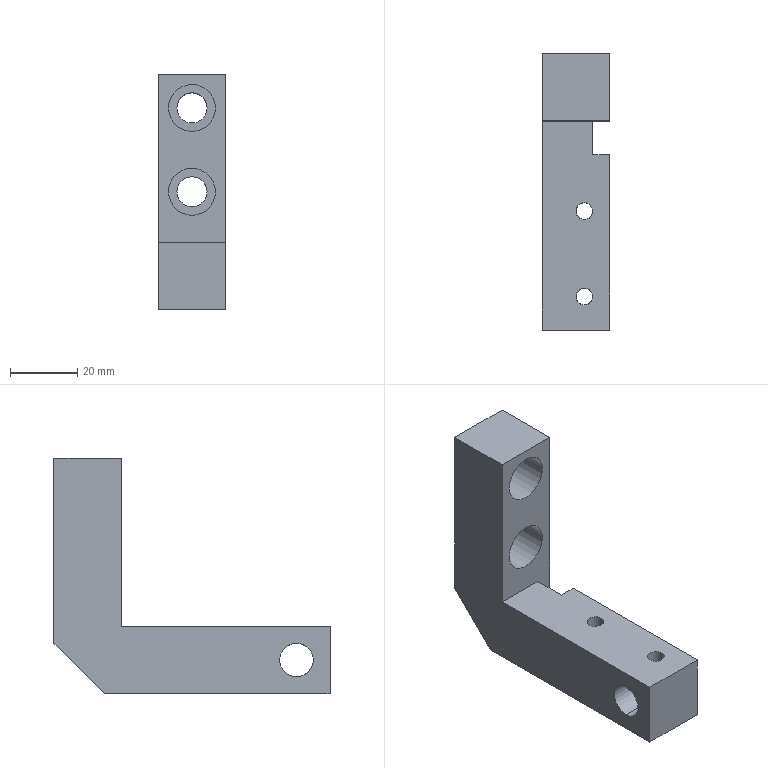Part | STEP file | Positioning_id2262_x_t | 1 solid | 35 faces | box 20 x 82.349 x 70.139 mm | volume 42004 mm3 | cylinder 20 | plane 15 | commonest cylinder face diameters 5 x8 9 x4 10 x4 14 x4